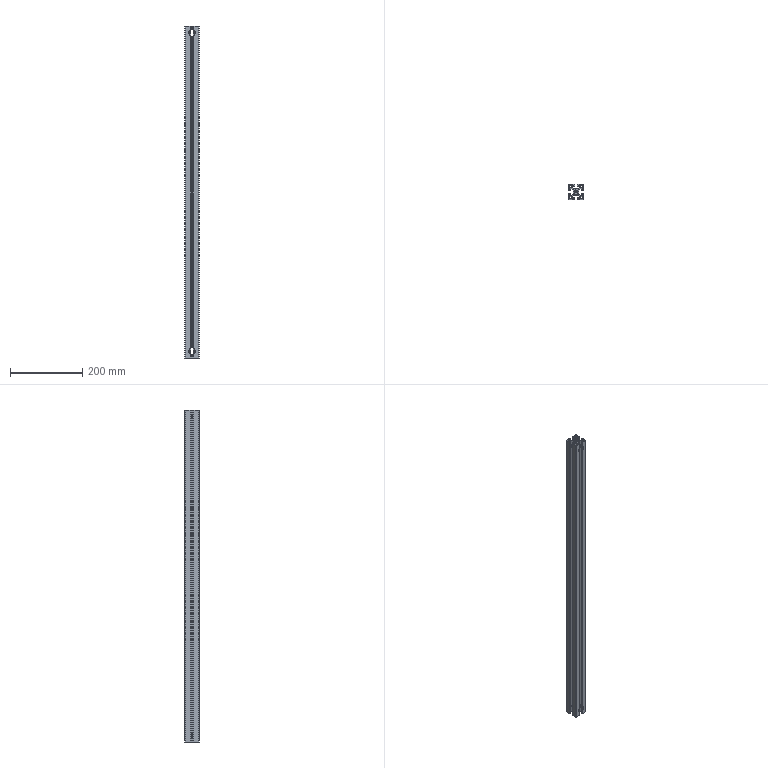Part | NX | features BREP 1 | 1 solid | 273 faces | box 40 x 40 x 920 mm | volume 552261 mm3 | plane 186 | cylinder 87 | commonest cylinder face diameters 1.5 x18 0.6 x16 2 x16 19 x16 6.8 x9 1 x8